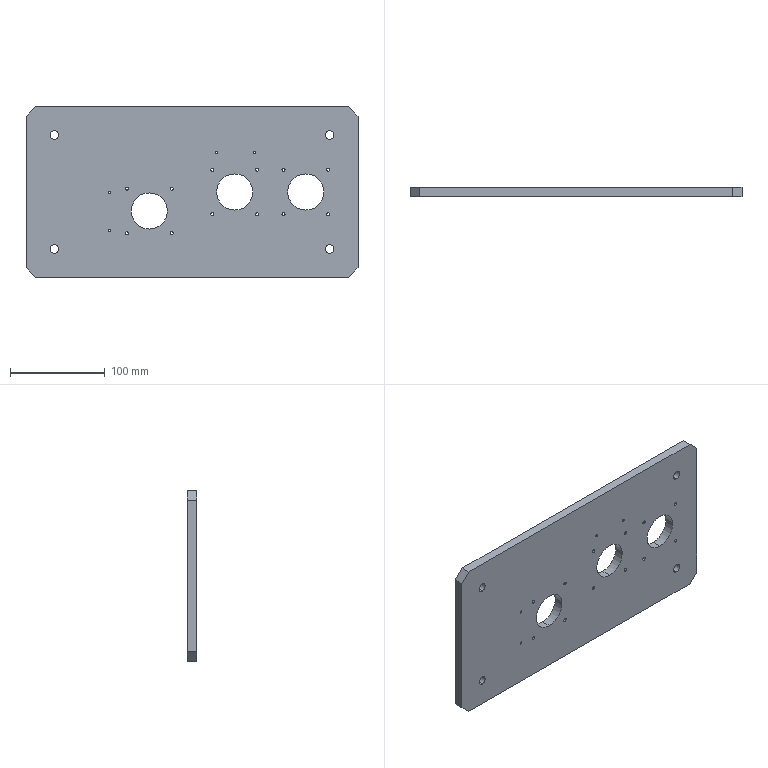Part | NX | features BREP 1 | 1 solid | 68 faces | box 350 x 10 x 180 mm | volume 587524 mm3 | cylinder 54 | plane 14 | commonest cylinder face diameters 3.3 x24 2.5 x8 9 x8 20 x8 38.1 x6